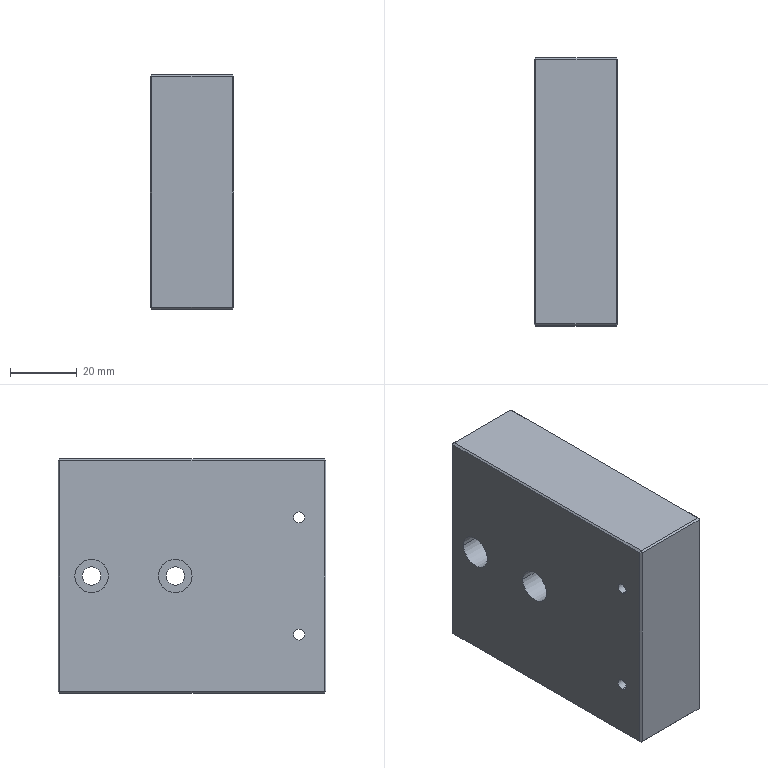Part | STEP file | 06-12 Driving feed slide plate | 1 solid | 56 faces | box 25 x 80 x 70 mm | volume 132614 mm3 | plane 41 | cylinder 15 | commonest cylinder face diameters 3.3 x4 5.5 x4 10 x4 2 x3